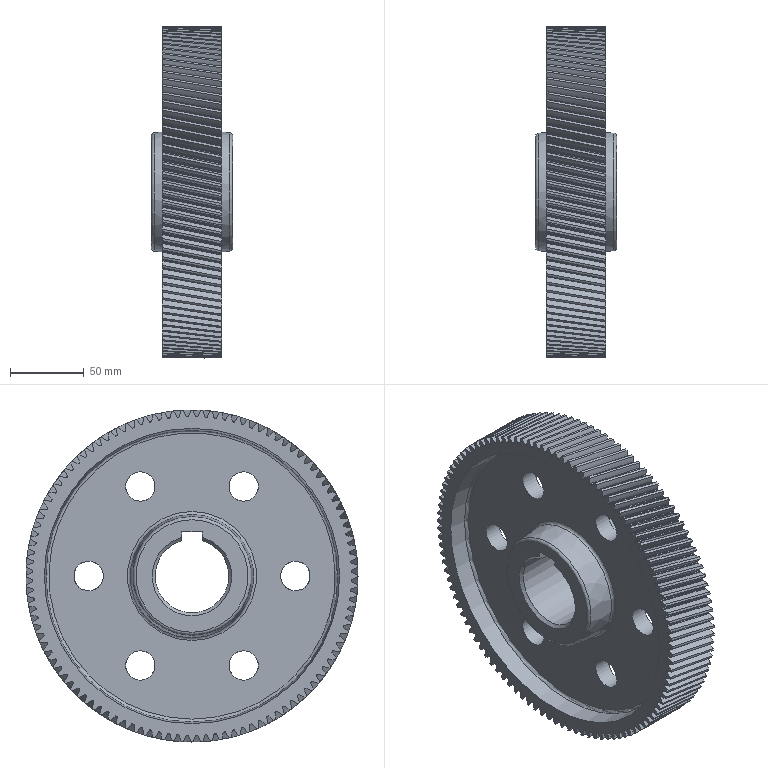Part | NX | features BREP 108, META 108, DATUM_CSYS 9, EXTRUDE 8, SKETCH 8, EXTRACT_DATUM_AXIS 6, DRAFT 4, BLEND 2, CHAMFER 2, EXTRACT_DATUM_PLANE 2, EXTRACT_FACE 2, EXTRACT_STRING 2, CYLINDER 1, DATUM_PLANE 1, FSET 1, Instance Feature 1, Mirror Feature 1 | 1 solid | 676 faces | box 55 x 224.908 x 224.908 mm | volume 752856 mm3 | spline 540 | cylinder 115 | plane 9 | cone 6 | torus 6 | commonest cylinder face diameters 215.908 x108 20 x6 50 x1